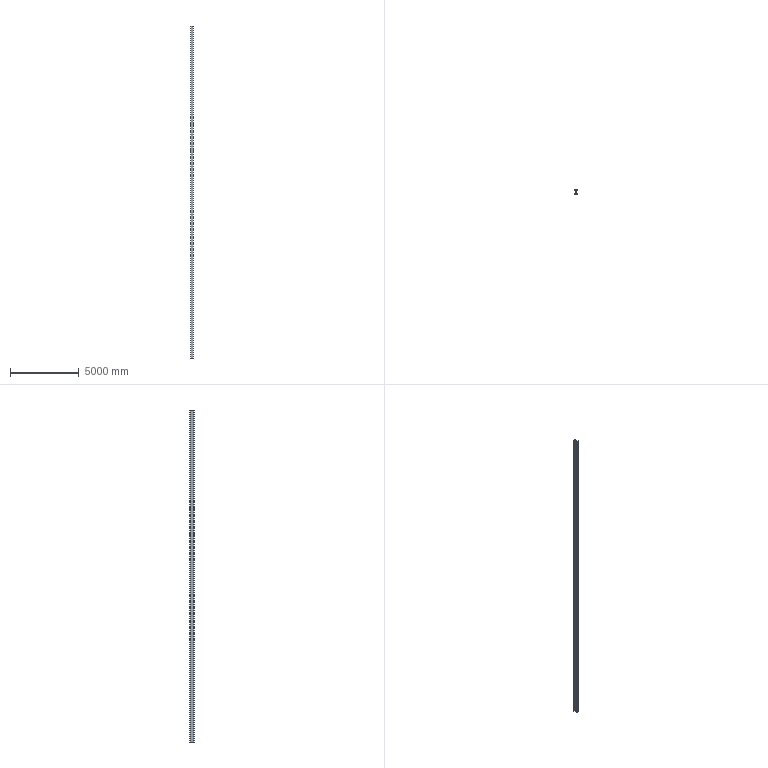Part | SolidWorks | features Extrusion 1 | 1 solid | 18 faces | box 150 x 300 x 24174 mm | volume 113087685 mm3 | plane 14 | cylinder 4 | commonest cylinder face diameters 26 x4
STEP:
#1=CARTESIAN_POINT('',(-75.,9.,0.));
#2=VERTEX_POINT('',#1);
#3=CARTESIAN_POINT('',(-75.,0.,0.));
#4=VERTEX_POINT('',#3);
#5=CARTESIAN_POINT('',(-75.,0.,0.));
#6=DIRECTION('',(0.,-1.,0.));
#7=VECTOR('',#6,1000.);
#8=LINE('',#5,#7);
#9=EDGE_CURVE('',#2,#4,#8,.T.);
#10=ORIENTED_EDGE('',*,*,#9,.T.);
#11=CARTESIAN_POINT('',(-75.,0.,24174.));
#12=VERTEX_POINT('',#11);
#13=CARTESIAN_POINT('',(-75.,0.,24174.));
#14=DIRECTION('',(0.,0.,-1.));
#15=VECTOR('',#14,1000.);
#16=LINE('',#13,#15);
#17=EDGE_CURVE('',#12,#4,#16,.T.);
#18=ORIENTED_EDGE('',*,*,#17,.F.);
#19=CARTESIAN_POINT('',(-75.,9.,24174.));
#20=VERTEX_POINT('',#19);
#21=CARTESIAN_POINT('',(-75.,0.,24174.));
#22=DIRECTION('',(0.,-1.,0.));
#23=VECTOR('',#22,1000.);
#24=LINE('',#21,#23);
#25=EDGE_CURVE('',#20,#12,#24,.T.);
#26=ORIENTED_EDGE('',*,*,#25,.F.);
#27=CARTESIAN_POINT('',(-75.,9.,24174.));
#28=DIRECTION('',(0.,0.,-1.));
#29=VECTOR('',#28,1000.);
#30=LINE('',#27,#29);
#31=EDGE_CURVE('',#20,#2,#30,.T.);
#32=ORIENTED_EDGE('',*,*,#31,.T.);
#33=EDGE_LOOP('',(#10,#18,#26,#32));
#34=FACE_OUTER_BOUND('',#33,.T.);
#35=CARTESIAN_POINT('',(-75.,0.,24174.));
#36=DIRECTION('',(1.,0.,0.));
#37=DIRECTION('',(0.,0.,-1.));
#38=AXIS2_PLACEMENT_3D('',#35,#36,#37);
#39=PLANE('',#38);
#40=ADVANCED_FACE('',(#34),#39,.F.);
#41=CARTESIAN_POINT('',(75.,0.,0.));
#42=VERTEX_POINT('',#41);
#43=CARTESIAN_POINT('',(75.,0.,0.));
#44=DIRECTION('',(1.,0.,0.));
#45=VECTOR('',#44,1000.);
#46=LINE('',#43,#45);
#47=EDGE_CURVE('',#4,#42,#46,.T.);
#48=ORIENTED_EDGE('',*,*,#47,.T.);
#49=CARTESIAN_POINT('',(75.,0.,24174.));
#50=VERTEX_POINT('',#49);
#51=CARTESIAN_POINT('',(75.,0.,24174.));
#52=DIRECTION('',(0.,0.,-1.));
#53=VECTOR('',#52,1000.);
#54=LINE('',#51,#53);
#55=EDGE_CURVE('',#50,#42,#54,.T.);
#56=ORIENTED_EDGE('',*,*,#55,.F.);
#57=CARTESIAN_POINT('',(75.,0.,24174.));
#58=DIRECTION('',(1.,0.,0.));
#59=VECTOR('',#58,1000.);
#60=LINE('',#57,#59);
#61=EDGE_CURVE('',#12,#50,#60,.T.);
#62=ORIENTED_EDGE('',*,*,#61,.F.);
#63=ORIENTED_EDGE('',*,*,#17,.T.);
#64=EDGE_LOOP('',(#48,#56,#62,#63));
#65=FACE_OUTER_BOUND('',#64,.T.);
#66=CARTESIAN_POINT('',(75.,0.,24174.));
#67=DIRECTION('',(0.,1.,0.));
#68=DIRECTION('',(-1.,0.,0.));
#69=AXIS2_PLACEMENT_3D('',#66,#67,#68);
#70=PLANE('',#69);
#71=ADVANCED_FACE('',(#65),#70,.F.);
#72=CARTESIAN_POINT('',(75.,9.,0.));
#73=VERTEX_POINT('',#72);
#74=CARTESIAN_POINT('',(75.,0.,0.));
#75=DIRECTION('',(0.,1.,0.));
#76=VECTOR('',#75,1000.);
#77=LINE('',#74,#76);
#78=EDGE_CURVE('',#42,#73,#77,.T.);
#79=ORIENTED_EDGE('',*,*,#78,.T.);
#80=CARTESIAN_POINT('',(75.,9.,24174.));
#81=VERTEX_POINT('',#80);
#82=CARTESIAN_POINT('',(75.,9.,24174.));
#83=DIRECTION('',(0.,0.,-1.));
#84=VECTOR('',#83,1000.);
#85=LINE('',#82,#84);
#86=EDGE_CURVE('',#81,#73,#85,.T.);
#87=ORIENTED_EDGE('',*,*,#86,.F.);
#88=CARTESIAN_POINT('',(75.,0.,24174.));
#89=DIRECTION('',(0.,1.,0.));
#90=VECTOR('',#89,1000.);
#91=LINE('',#88,#90);
#92=EDGE_CURVE('',#50,#81,#91,.T.);
#93=ORIENTED_EDGE('',*,*,#92,.F.);
#94=ORIENTED_EDGE('',*,*,#55,.T.);
#95=EDGE_LOOP('',(#79,#87,#93,#94));
#96=FACE_OUTER_BOUND('',#95,.T.);
#97=CARTESIAN_POINT('',(75.,0.,24174.));
#98=DIRECTION('',(-1.,0.,0.));
#99=DIRECTION('',(0.,0.,1.));
#100=AXIS2_PLACEMENT_3D('',#97,#98,#99);
#101=PLANE('',#100);
#102=ADVANCED_FACE('',(#96),#101,.F.);
#103=CARTESIAN_POINT('',(16.25,9.,0.));
#104=VERTEX_POINT('',#103);
#105=CARTESIAN_POINT('',(75.,9.,0.));
#106=DIRECTION('',(-1.,0.,0.));
#107=VECTOR('',#106,1000.);
#108=LINE('',#105,#107);
#109=EDGE_CURVE('',#73,#104,#108,.T.);
#110=ORIENTED_EDGE('',*,*,#109,.T.);
#111=CARTESIAN_POINT('',(16.25,9.,24174.));
#112=VERTEX_POINT('',#111);
#113=CARTESIAN_POINT('',(16.25,9.,24174.));
#114=DIRECTION('',(0.,0.,-1.));
#115=VECTOR('',#114,1000.);
#116=LINE('',#113,#115);
#117=EDGE_CURVE('',#112,#104,#116,.T.);
#118=ORIENTED_EDGE('',*,*,#117,.F.);
#119=CARTESIAN_POINT('',(75.,9.,24174.));
#120=DIRECTION('',(-1.,0.,0.));
#121=VECTOR('',#120,1000.);
#122=LINE('',#119,#121);
#123=EDGE_CURVE('',#81,#112,#122,.T.);
#124=ORIENTED_EDGE('',*,*,#123,.F.);
#125=ORIENTED_EDGE('',*,*,#86,.T.);
#126=EDGE_LOOP('',(#110,#118,#124,#125));
#127=FACE_OUTER_BOUND('',#126,.T.);
#128=CARTESIAN_POINT('',(75.,9.,24174.));
#129=DIRECTION('',(0.,-1.,0.));
#130=DIRECTION('',(1.,0.,0.));
#131=AXIS2_PLACEMENT_3D('',#128,#129,#130);
#132=PLANE('',#131);
#133=ADVANCED_FACE('',(#127),#132,.F.);
#134=CARTESIAN_POINT('',(3.25,22.,0.));
#135=VERTEX_POINT('',#134);
#136=CARTESIAN_POINT('',(16.25,22.,0.));
#137=DIRECTION('',(0.,0.,-1.));
#138=DIRECTION('',(-1.,0.,0.));
#139=AXIS2_PLACEMENT_3D('',#136,#137,#138);
#140=CIRCLE('',#139,13.);
#141=EDGE_CURVE('',#104,#135,#140,.T.);
#142=ORIENTED_EDGE('',*,*,#141,.T.);
#143=CARTESIAN_POINT('',(3.25,22.,24174.));
#144=VERTEX_POINT('',#143);
#145=CARTESIAN_POINT('',(3.25,22.,24174.));
#146=DIRECTION('',(0.,0.,-1.));
#147=VECTOR('',#146,1000.);
#148=LINE('',#145,#147);
#149=EDGE_CURVE('',#144,#135,#148,.T.);
#150=ORIENTED_EDGE('',*,*,#149,.F.);
#151=CARTESIAN_POINT('',(16.25,22.,24174.));
#152=DIRECTION('',(0.,0.,-1.));
#153=DIRECTION('',(-1.,0.,0.));
#154=AXIS2_PLACEMENT_3D('',#151,#152,#153);
#155=CIRCLE('',#154,13.);
#156=EDGE_CURVE('',#112,#144,#155,.T.);
#157=ORIENTED_EDGE('',*,*,#156,.F.);
#158=ORIENTED_EDGE('',*,*,#117,.T.);
#159=EDGE_LOOP('',(#142,#150,#157,#158));
#160=FACE_OUTER_BOUND('',#159,.T.);
#161=CARTESIAN_POINT('',(16.25,22.,24174.));
#162=DIRECTION('',(0.,0.,-1.));
#163=DIRECTION('',(-1.,0.,0.));
#164=AXIS2_PLACEMENT_3D('',#161,#162,#163);
#165=CYLINDRICAL_SURFACE('',#164,13.);
#166=ADVANCED_FACE('',(#160),#165,.F.);
#167=CARTESIAN_POINT('',(3.25,278.,0.));
#168=VERTEX_POINT('',#167);
#169=CARTESIAN_POINT('',(3.25,22.,0.));
#170=DIRECTION('',(0.,1.,0.));
#171=VECTOR('',#170,1000.);
#172=LINE('',#169,#171);
#173=EDGE_CURVE('',#135,#168,#172,.T.);
#174=ORIENTED_EDGE('',*,*,#173,.T.);
#175=CARTESIAN_POINT('',(3.25,278.,24174.));
#176=VERTEX_POINT('',#175);
#177=CARTESIAN_POINT('',(3.25,278.,24174.));
#178=DIRECTION('',(0.,0.,-1.));
#179=VECTOR('',#178,1000.);
#180=LINE('',#177,#179);
#181=EDGE_CURVE('',#176,#168,#180,.T.);
#182=ORIENTED_EDGE('',*,*,#181,.F.);
#183=CARTESIAN_POINT('',(3.25,22.,24174.));
#184=DIRECTION('',(0.,1.,0.));
#185=VECTOR('',#184,1000.);
#186=LINE('',#183,#185);
#187=EDGE_CURVE('',#144,#176,#186,.T.);
#188=ORIENTED_EDGE('',*,*,#187,.F.);
#189=ORIENTED_EDGE('',*,*,#149,.T.);
#190=EDGE_LOOP('',(#174,#182,#188,#189));
#191=FACE_OUTER_BOUND('',#190,.T.);
#192=CARTESIAN_POINT('',(3.25,22.,24174.));
#193=DIRECTION('',(-1.,0.,0.));
#194=DIRECTION('',(0.,0.,1.));
#195=AXIS2_PLACEMENT_3D('',#192,#193,#194);
#196=PLANE('',#195);
#197=ADVANCED_FACE('',(#191),#196,.F.);
#198=CARTESIAN_POINT('',(16.25,291.,0.));
#199=VERTEX_POINT('',#198);
#200=CARTESIAN_POINT('',(16.25,278.,0.));
#201=DIRECTION('',(0.,0.,-1.));
#202=DIRECTION('',(-1.,0.,0.));
#203=AXIS2_PLACEMENT_3D('',#200,#201,#202);
#204=CIRCLE('',#203,13.);
#205=EDGE_CURVE('',#168,#199,#204,.T.);
#206=ORIENTED_EDGE('',*,*,#205,.T.);
#207=CARTESIAN_POINT('',(16.25,291.,24174.));
#208=VERTEX_POINT('',#207);
#209=CARTESIAN_POINT('',(16.25,291.,24174.));
#210=DIRECTION('',(0.,0.,-1.));
#211=VECTOR('',#210,1000.);
#212=LINE('',#209,#211);
#213=EDGE_CURVE('',#208,#199,#212,.T.);
#214=ORIENTED_EDGE('',*,*,#213,.F.);
#215=CARTESIAN_POINT('',(16.25,278.,24174.));
#216=DIRECTION('',(0.,0.,-1.));
#217=DIRECTION('',(-1.,0.,0.));
#218=AXIS2_PLACEMENT_3D('',#215,#216,#217);
#219=CIRCLE('',#218,13.);
#220=EDGE_CURVE('',#176,#208,#219,.T.);
#221=ORIENTED_EDGE('',*,*,#220,.F.);
#222=ORIENTED_EDGE('',*,*,#181,.T.);
#223=EDGE_LOOP('',(#206,#214,#221,#222));
#224=FACE_OUTER_BOUND('',#223,.T.);
#225=CARTESIAN_POINT('',(16.25,278.,24174.));
#226=DIRECTION('',(0.,0.,-1.));
#227=DIRECTION('',(-1.,0.,0.));
#228=AXIS2_PLACEMENT_3D('',#225,#226,#227);
#229=CYLINDRICAL_SURFACE('',#228,13.);
#230=ADVANCED_FACE('',(#224),#229,.F.);
#231=CARTESIAN_POINT('',(75.,291.,0.));
#232=VERTEX_POINT('',#231);
#233=CARTESIAN_POINT('',(16.25,291.,0.));
#234=DIRECTION('',(1.,0.,0.));
#235=VECTOR('',#234,1000.);
#236=LINE('',#233,#235);
#237=EDGE_CURVE('',#199,#232,#236,.T.);
#238=ORIENTED_EDGE('',*,*,#237,.T.);
#239=CARTESIAN_POINT('',(75.,291.,24174.));
#240=VERTEX_POINT('',#239);
#241=CARTESIAN_POINT('',(75.,291.,24174.));
#242=DIRECTION('',(0.,0.,-1.));
#243=VECTOR('',#242,1000.);
#244=LINE('',#241,#243);
#245=EDGE_CURVE('',#240,#232,#244,.T.);
#246=ORIENTED_EDGE('',*,*,#245,.F.);
#247=CARTESIAN_POINT('',(16.25,291.,24174.));
#248=DIRECTION('',(1.,0.,0.));
#249=VECTOR('',#248,1000.);
#250=LINE('',#247,#249);
#251=EDGE_CURVE('',#208,#240,#250,.T.);
#252=ORIENTED_EDGE('',*,*,#251,.F.);
#253=ORIENTED_EDGE('',*,*,#213,.T.);
#254=EDGE_LOOP('',(#238,#246,#252,#253));
#255=FACE_OUTER_BOUND('',#254,.T.);
#256=CARTESIAN_POINT('',(16.25,291.,24174.));
#257=DIRECTION('',(0.,1.,0.));
#258=DIRECTION('',(-1.,0.,0.));
#259=AXIS2_PLACEMENT_3D('',#256,#257,#258);
#260=PLANE('',#259);
#261=ADVANCED_FACE('',(#255),#260,.F.);
#262=CARTESIAN_POINT('',(75.,300.,0.));
#263=VERTEX_POINT('',#262);
#264=CARTESIAN_POINT('',(75.,291.,0.));
#265=DIRECTION('',(0.,1.,0.));
#266=VECTOR('',#265,1000.);
#267=LINE('',#264,#266);
#268=EDGE_CURVE('',#232,#263,#267,.T.);
#269=ORIENTED_EDGE('',*,*,#268,.T.);
#270=CARTESIAN_POINT('',(75.,300.,24174.));
#271=VERTEX_POINT('',#270);
#272=CARTESIAN_POINT('',(75.,300.,24174.));
#273=DIRECTION('',(0.,0.,-1.));
#274=VECTOR('',#273,1000.);
#275=LINE('',#272,#274);
#276=EDGE_CURVE('',#271,#263,#275,.T.);
#277=ORIENTED_EDGE('',*,*,#276,.F.);
#278=CARTESIAN_POINT('',(75.,291.,24174.));
#279=DIRECTION('',(0.,1.,0.));
#280=VECTOR('',#279,1000.);
#281=LINE('',#278,#280);
#282=EDGE_CURVE('',#240,#271,#281,.T.);
#283=ORIENTED_EDGE('',*,*,#282,.F.);
#284=ORIENTED_EDGE('',*,*,#245,.T.);
#285=EDGE_LOOP('',(#269,#277,#283,#284));
#286=FACE_OUTER_BOUND('',#285,.T.);
#287=CARTESIAN_POINT('',(75.,291.,24174.));
#288=DIRECTION('',(-1.,0.,0.));
#289=DIRECTION('',(0.,-1.,0.));
#290=AXIS2_PLACEMENT_3D('',#287,#288,#289);
#291=PLANE('',#290);
#292=ADVANCED_FACE('',(#286),#291,.F.);
#293=CARTESIAN_POINT('',(-75.,300.,0.));
#294=VERTEX_POINT('',#293);
#295=CARTESIAN_POINT('',(-75.,300.,0.));
#296=DIRECTION('',(-1.,0.,0.));
#297=VECTOR('',#296,1000.);
#298=LINE('',#295,#297);
#299=EDGE_CURVE('',#263,#294,#298,.T.);
#300=ORIENTED_EDGE('',*,*,#299,.T.);
#301=CARTESIAN_POINT('',(-75.,300.,24174.));
#302=VERTEX_POINT('',#301);
#303=CARTESIAN_POINT('',(-75.,300.,24174.));
#304=DIRECTION('',(0.,0.,-1.));
#305=VECTOR('',#304,1000.);
#306=LINE('',#303,#305);
#307=EDGE_CURVE('',#302,#294,#306,.T.);
#308=ORIENTED_EDGE('',*,*,#307,.F.);
#309=CARTESIAN_POINT('',(-75.,300.,24174.));
#310=DIRECTION('',(-1.,0.,0.));
#311=VECTOR('',#310,1000.);
#312=LINE('',#309,#311);
#313=EDGE_CURVE('',#271,#302,#312,.T.);
#314=ORIENTED_EDGE('',*,*,#313,.F.);
#315=ORIENTED_EDGE('',*,*,#276,.T.);
#316=EDGE_LOOP('',(#300,#308,#314,#315));
#317=FACE_OUTER_BOUND('',#316,.T.);
#318=CARTESIAN_POINT('',(-75.,300.,24174.));
#319=DIRECTION('',(0.,-1.,0.));
#320=DIRECTION('',(0.,0.,-1.));
#321=AXIS2_PLACEMENT_3D('',#318,#319,#320);
#322=PLANE('',#321);
#323=ADVANCED_FACE('',(#317),#322,.F.);
#324=CARTESIAN_POINT('',(-75.,291.,0.));
#325=VERTEX_POINT('',#324);
#326=CARTESIAN_POINT('',(-75.,291.,0.));
#327=DIRECTION('',(0.,-1.,0.));
#328=VECTOR('',#327,1000.);
#329=LINE('',#326,#328);
#330=EDGE_CURVE('',#294,#325,#329,.T.);
#331=ORIENTED_EDGE('',*,*,#330,.T.);
#332=CARTESIAN_POINT('',(-75.,291.,24174.));
#333=VERTEX_POINT('',#332);
#334=CARTESIAN_POINT('',(-75.,291.,24174.));
#335=DIRECTION('',(0.,0.,-1.));
#336=VECTOR('',#335,1000.);
#337=LINE('',#334,#336);
#338=EDGE_CURVE('',#333,#325,#337,.T.);
#339=ORIENTED_EDGE('',*,*,#338,.F.);
#340=CARTESIAN_POINT('',(-75.,291.,24174.));
#341=DIRECTION('',(0.,-1.,0.));
#342=VECTOR('',#341,1000.);
#343=LINE('',#340,#342);
#344=EDGE_CURVE('',#302,#333,#343,.T.);
#345=ORIENTED_EDGE('',*,*,#344,.F.);
#346=ORIENTED_EDGE('',*,*,#307,.T.);
#347=EDGE_LOOP('',(#331,#339,#345,#346));
#348=FACE_OUTER_BOUND('',#347,.T.);
#349=CARTESIAN_POINT('',(-75.,291.,24174.));
#350=DIRECTION('',(1.,0.,0.));
#351=DIRECTION('',(0.,1.,0.));
#352=AXIS2_PLACEMENT_3D('',#349,#350,#351);
#353=PLANE('',#352);
#354=ADVANCED_FACE('',(#348),#353,.F.);
#355=CARTESIAN_POINT('',(-16.25,291.,0.));
#356=VERTEX_POINT('',#355);
#357=CARTESIAN_POINT('',(-16.25,291.,0.));
#358=DIRECTION('',(1.,0.,0.));
#359=VECTOR('',#358,1000.);
#360=LINE('',#357,#359);
#361=EDGE_CURVE('',#325,#356,#360,.T.);
#362=ORIENTED_EDGE('',*,*,#361,.T.);
#363=CARTESIAN_POINT('',(-16.25,291.,24174.));
#364=VERTEX_POINT('',#363);
#365=CARTESIAN_POINT('',(-16.25,291.,24174.));
#366=DIRECTION('',(0.,0.,-1.));
#367=VECTOR('',#366,1000.);
#368=LINE('',#365,#367);
#369=EDGE_CURVE('',#364,#356,#368,.T.);
#370=ORIENTED_EDGE('',*,*,#369,.F.);
#371=CARTESIAN_POINT('',(-16.25,291.,24174.));
#372=DIRECTION('',(1.,0.,0.));
#373=VECTOR('',#372,1000.);
#374=LINE('',#371,#373);
#375=EDGE_CURVE('',#333,#364,#374,.T.);
#376=ORIENTED_EDGE('',*,*,#375,.F.);
#377=ORIENTED_EDGE('',*,*,#338,.T.);
#378=EDGE_LOOP('',(#362,#370,#376,#377));
#379=FACE_OUTER_BOUND('',#378,.T.);
#380=CARTESIAN_POINT('',(-16.25,291.,24174.));
#381=DIRECTION('',(0.,1.,0.));
#382=DIRECTION('',(-1.,0.,0.));
#383=AXIS2_PLACEMENT_3D('',#380,#381,#382);
#384=PLANE('',#383);
#385=ADVANCED_FACE('',(#379),#384,.F.);
#386=CARTESIAN_POINT('',(-3.25,278.,0.));
#387=VERTEX_POINT('',#386);
#388=CARTESIAN_POINT('',(-16.25,278.,0.));
#389=DIRECTION('',(0.,0.,-1.));
#390=DIRECTION('',(1.,0.,0.));
#391=AXIS2_PLACEMENT_3D('',#388,#389,#390);
#392=CIRCLE('',#391,13.);
#393=EDGE_CURVE('',#356,#387,#392,.T.);
#394=ORIENTED_EDGE('',*,*,#393,.T.);
#395=CARTESIAN_POINT('',(-3.25,278.,24174.));
#396=VERTEX_POINT('',#395);
#397=CARTESIAN_POINT('',(-3.25,278.,24174.));
#398=DIRECTION('',(0.,0.,-1.));
#399=VECTOR('',#398,1000.);
#400=LINE('',#397,#399);
#401=EDGE_CURVE('',#396,#387,#400,.T.);
#402=ORIENTED_EDGE('',*,*,#401,.F.);
#403=CARTESIAN_POINT('',(-16.25,278.,24174.));
#404=DIRECTION('',(0.,0.,-1.));
#405=DIRECTION('',(1.,0.,0.));
#406=AXIS2_PLACEMENT_3D('',#403,#404,#405);
#407=CIRCLE('',#406,13.);
#408=EDGE_CURVE('',#364,#396,#407,.T.);
#409=ORIENTED_EDGE('',*,*,#408,.F.);
#410=ORIENTED_EDGE('',*,*,#369,.T.);
#411=EDGE_LOOP('',(#394,#402,#409,#410));
#412=FACE_OUTER_BOUND('',#411,.T.);
#413=CARTESIAN_POINT('',(-16.25,278.,24174.));
#414=DIRECTION('',(0.,0.,-1.));
#415=DIRECTION('',(-1.,0.,0.));
#416=AXIS2_PLACEMENT_3D('',#413,#414,#415);
#417=CYLINDRICAL_SURFACE('',#416,13.);
#418=ADVANCED_FACE('',(#412),#417,.F.);
#419=CARTESIAN_POINT('',(-3.25,22.,0.));
#420=VERTEX_POINT('',#419);
#421=CARTESIAN_POINT('',(-3.25,22.,0.));
#422=DIRECTION('',(0.,-1.,0.));
#423=VECTOR('',#422,1000.);
#424=LINE('',#421,#423);
#425=EDGE_CURVE('',#387,#420,#424,.T.);
#426=ORIENTED_EDGE('',*,*,#425,.T.);
#427=CARTESIAN_POINT('',(-3.25,22.,24174.));
#428=VERTEX_POINT('',#427);
#429=CARTESIAN_POINT('',(-3.25,22.,24174.));
#430=DIRECTION('',(0.,0.,-1.));
#431=VECTOR('',#430,1000.);
#432=LINE('',#429,#431);
#433=EDGE_CURVE('',#428,#420,#432,.T.);
#434=ORIENTED_EDGE('',*,*,#433,.F.);
#435=CARTESIAN_POINT('',(-3.25,22.,24174.));
#436=DIRECTION('',(0.,-1.,0.));
#437=VECTOR('',#436,1000.);
#438=LINE('',#435,#437);
#439=EDGE_CURVE('',#396,#428,#438,.T.);
#440=ORIENTED_EDGE('',*,*,#439,.F.);
#441=ORIENTED_EDGE('',*,*,#401,.T.);
#442=EDGE_LOOP('',(#426,#434,#440,#441));
#443=FACE_OUTER_BOUND('',#442,.T.);
#444=CARTESIAN_POINT('',(-3.25,22.,24174.));
#445=DIRECTION('',(1.,0.,0.));
#446=DIRECTION('',(0.,0.,-1.));
#447=AXIS2_PLACEMENT_3D('',#444,#445,#446);
#448=PLANE('',#447);
#449=ADVANCED_FACE('',(#443),#448,.F.);
#450=CARTESIAN_POINT('',(-16.25,9.,0.));
#451=VERTEX_POINT('',#450);
#452=CARTESIAN_POINT('',(-16.25,22.,0.));
#453=DIRECTION('',(0.,0.,-1.));
#454=DIRECTION('',(-1.,0.,0.));
#455=AXIS2_PLACEMENT_3D('',#452,#453,#454);
#456=CIRCLE('',#455,13.);
#457=EDGE_CURVE('',#420,#451,#456,.T.);
#458=ORIENTED_EDGE('',*,*,#457,.T.);
#459=CARTESIAN_POINT('',(-16.25,9.,24174.));
#460=VERTEX_POINT('',#459);
#461=CARTESIAN_POINT('',(-16.25,9.,24174.));
#462=DIRECTION('',(0.,0.,-1.));
#463=VECTOR('',#462,1000.);
#464=LINE('',#461,#463);
#465=EDGE_CURVE('',#460,#451,#464,.T.);
#466=ORIENTED_EDGE('',*,*,#465,.F.);
#467=CARTESIAN_POINT('',(-16.25,22.,24174.));
#468=DIRECTION('',(0.,0.,-1.));
#469=DIRECTION('',(-1.,0.,0.));
#470=AXIS2_PLACEMENT_3D('',#467,#468,#469);
#471=CIRCLE('',#470,13.);
#472=EDGE_CURVE('',#428,#460,#471,.T.);
#473=ORIENTED_EDGE('',*,*,#472,.F.);
#474=ORIENTED_EDGE('',*,*,#433,.T.);
#475=EDGE_LOOP('',(#458,#466,#473,#474));
#476=FACE_OUTER_BOUND('',#475,.T.);
#477=CARTESIAN_POINT('',(-16.25,22.,24174.));
#478=DIRECTION('',(0.,0.,-1.));
#479=DIRECTION('',(-1.,0.,0.));
#480=AXIS2_PLACEMENT_3D('',#477,#478,#479);
#481=CYLINDRICAL_SURFACE('',#480,13.);
#482=ADVANCED_FACE('',(#476),#481,.F.);
#483=CARTESIAN_POINT('',(-75.,9.,0.));
#484=DIRECTION('',(-1.,0.,0.));
#485=VECTOR('',#484,1000.);
#486=LINE('',#483,#485);
#487=EDGE_CURVE('',#451,#2,#486,.T.);
#488=ORIENTED_EDGE('',*,*,#487,.T.);
#489=ORIENTED_EDGE('',*,*,#31,.F.);
#490=CARTESIAN_POINT('',(-75.,9.,24174.));
#491=DIRECTION('',(-1.,0.,0.));
#492=VECTOR('',#491,1000.);
#493=LINE('',#490,#492);
#494=EDGE_CURVE('',#460,#20,#493,.T.);
#495=ORIENTED_EDGE('',*,*,#494,.F.);
#496=ORIENTED_EDGE('',*,*,#465,.T.);
#497=EDGE_LOOP('',(#488,#489,#495,#496));
#498=FACE_OUTER_BOUND('',#497,.T.);
#499=CARTESIAN_POINT('',(-75.,9.,24174.));
#500=DIRECTION('',(0.,-1.,0.));
#501=DIRECTION('',(1.,0.,0.));
#502=AXIS2_PLACEMENT_3D('',#499,#500,#501);
#503=PLANE('',#502);
#504=ADVANCED_FACE('',(#498),#503,.F.);
#505=ORIENTED_EDGE('',*,*,#25,.T.);
#506=ORIENTED_EDGE('',*,*,#61,.T.);
#507=ORIENTED_EDGE('',*,*,#92,.T.);
#508=ORIENTED_EDGE('',*,*,#123,.T.);
#509=ORIENTED_EDGE('',*,*,#156,.T.);
#510=ORIENTED_EDGE('',*,*,#187,.T.);
#511=ORIENTED_EDGE('',*,*,#220,.T.);
#512=ORIENTED_EDGE('',*,*,#251,.T.);
#513=ORIENTED_EDGE('',*,*,#282,.T.);
#514=ORIENTED_EDGE('',*,*,#313,.T.);
#515=ORIENTED_EDGE('',*,*,#344,.T.);
#516=ORIENTED_EDGE('',*,*,#375,.T.);
#517=ORIENTED_EDGE('',*,*,#408,.T.);
#518=ORIENTED_EDGE('',*,*,#439,.T.);
#519=ORIENTED_EDGE('',*,*,#472,.T.);
#520=ORIENTED_EDGE('',*,*,#494,.T.);
#521=EDGE_LOOP('',(#505,#506,#507,#508,#509,#510,#511,#512,#513,#514,#515,#516,#517,#518,#519,#520));
#522=FACE_OUTER_BOUND('',#521,.T.);
#523=CARTESIAN_POINT('',(-16.25,22.,24174.));
#524=DIRECTION('',(0.,0.,-1.));
#525=DIRECTION('',(-1.,0.,0.));
#526=AXIS2_PLACEMENT_3D('',#523,#524,#525);
#527=PLANE('',#526);
#528=ADVANCED_FACE('',(#522),#527,.F.);
#529=ORIENTED_EDGE('',*,*,#9,.F.);
#530=ORIENTED_EDGE('',*,*,#487,.F.);
#531=ORIENTED_EDGE('',*,*,#457,.F.);
#532=ORIENTED_EDGE('',*,*,#425,.F.);
#533=ORIENTED_EDGE('',*,*,#393,.F.);
#534=ORIENTED_EDGE('',*,*,#361,.F.);
#535=ORIENTED_EDGE('',*,*,#330,.F.);
#536=ORIENTED_EDGE('',*,*,#299,.F.);
#537=ORIENTED_EDGE('',*,*,#268,.F.);
#538=ORIENTED_EDGE('',*,*,#237,.F.);
#539=ORIENTED_EDGE('',*,*,#205,.F.);
#540=ORIENTED_EDGE('',*,*,#173,.F.);
#541=ORIENTED_EDGE('',*,*,#141,.F.);
#542=ORIENTED_EDGE('',*,*,#109,.F.);
#543=ORIENTED_EDGE('',*,*,#78,.F.);
#544=ORIENTED_EDGE('',*,*,#47,.F.);
#545=EDGE_LOOP('',(#529,#530,#531,#532,#533,#534,#535,#536,#537,#538,#539,#540,#541,#542,#543,#544));
#546=FACE_OUTER_BOUND('',#545,.T.);
#547=CARTESIAN_POINT('',(-16.25,22.,0.));
#548=DIRECTION('',(0.,0.,-1.));
#549=DIRECTION('',(-1.,0.,0.));
#550=AXIS2_PLACEMENT_3D('',#547,#548,#549);
#551=PLANE('',#550);
#552=ADVANCED_FACE('',(#546),#551,.T.);
#553=CLOSED_SHELL('',(#40,#71,#102,#133,#166,#197,#230,#261,#292,#323,#354,#385,#418,#449,#482,#504,#528,#552));
#554=MANIFOLD_SOLID_BREP('',#553);
#555=CARTESIAN_POINT('',(0.,0.,0.));
#556=DIRECTION('',(0.,0.,1.));
#557=DIRECTION('',(1.,0.,0.));
#558=AXIS2_PLACEMENT_3D('',#555,#556,#557);
#559=(LENGTH_UNIT()NAMED_UNIT(*)SI_UNIT(.MILLI.,.METRE.));
#560=UNCERTAINTY_MEASURE_WITH_UNIT(LENGTH_MEASURE(0.00001),#559,'','');
#561=(NAMED_UNIT(*)PLANE_ANGLE_UNIT()SI_UNIT($,.RADIAN.));
#562=(NAMED_UNIT(*)SI_UNIT($,.STERADIAN.)SOLID_ANGLE_UNIT());
#563=(GEOMETRIC_REPRESENTATION_CONTEXT(3)GLOBAL_UNCERTAINTY_ASSIGNED_CONTEXT((#560))GLOBAL_UNIT_ASSIGNED_CONTEXT((#559,#561,#562))REPRESENTATION_CONTEXT('',''));
#564=ADVANCED_BREP_SHAPE_REPRESENTATION('',(#554,#558),#563);